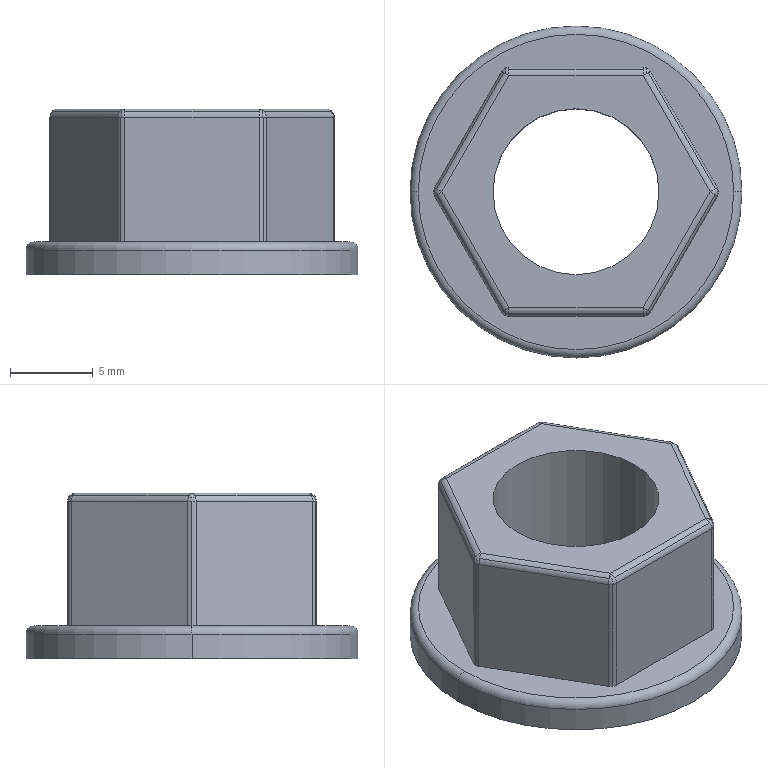Part | SolidWorks | features BaseBody 1 | 1 solid | 51 faces | box 20 x 20 x 10 mm | volume 1395 mm3 | cylinder 28 | sphere 12 | plane 9 | torus 2 | commonest cylinder face diameters 1 x24 10 x2 20 x2
STEP:
#1=CARTESIAN_POINT('',(-5.,0.,10.));
#2=VERTEX_POINT('',#1);
#3=CARTESIAN_POINT('',(5.,0.,10.));
#4=VERTEX_POINT('',#3);
#5=CARTESIAN_POINT('',(0.,0.,10.));
#6=DIRECTION('',(0.,0.,-1.));
#7=DIRECTION('',(1.,0.,0.));
#8=AXIS2_PLACEMENT_3D('',#5,#6,#7);
#9=CIRCLE('',#8,5.);
#10=EDGE_CURVE('',#2,#4,#9,.T.);
#11=ORIENTED_EDGE('',*,*,#10,.F.);
#12=CARTESIAN_POINT('',(-5.,0.,0.));
#13=VERTEX_POINT('',#12);
#14=CARTESIAN_POINT('',(-5.,0.,0.));
#15=DIRECTION('',(0.,0.,-1.));
#16=VECTOR('',#15,1000.);
#17=LINE('',#14,#16);
#18=EDGE_CURVE('',#2,#13,#17,.T.);
#19=ORIENTED_EDGE('',*,*,#18,.T.);
#20=CARTESIAN_POINT('',(5.,0.,0.));
#21=VERTEX_POINT('',#20);
#22=CARTESIAN_POINT('',(0.,0.,0.));
#23=DIRECTION('',(0.,0.,1.));
#24=DIRECTION('',(1.,0.,0.));
#25=AXIS2_PLACEMENT_3D('',#22,#23,#24);
#26=CIRCLE('',#25,5.);
#27=EDGE_CURVE('',#21,#13,#26,.T.);
#28=ORIENTED_EDGE('',*,*,#27,.F.);
#29=CARTESIAN_POINT('',(5.,0.,0.));
#30=DIRECTION('',(0.,0.,-1.));
#31=VECTOR('',#30,1000.);
#32=LINE('',#29,#31);
#33=EDGE_CURVE('',#4,#21,#32,.T.);
#34=ORIENTED_EDGE('',*,*,#33,.F.);
#35=EDGE_LOOP('',(#11,#19,#28,#34));
#36=FACE_OUTER_BOUND('',#35,.T.);
#37=CARTESIAN_POINT('',(0.,0.,0.));
#38=DIRECTION('',(0.,0.,-1.));
#39=DIRECTION('',(1.,0.,0.));
#40=AXIS2_PLACEMENT_3D('',#37,#38,#39);
#41=CYLINDRICAL_SURFACE('',#40,5.);
#42=ADVANCED_FACE('',(#36),#41,.F.);
#43=CARTESIAN_POINT('',(-4.227,-7.464,9.5));
#44=VERTEX_POINT('',#43);
#45=CARTESIAN_POINT('',(-4.291,-7.433,9.5));
#46=VERTEX_POINT('',#45);
#47=CARTESIAN_POINT('',(-4.041,-7.,9.5));
#48=DIRECTION('',(0.,0.,-1.));
#49=DIRECTION('',(0.,-1.,0.));
#50=AXIS2_PLACEMENT_3D('',#47,#48,#49);
#51=CIRCLE('',#50,0.5);
#52=EDGE_CURVE('',#44,#46,#51,.T.);
#53=ORIENTED_EDGE('',*,*,#52,.F.);
#54=CARTESIAN_POINT('',(-4.202,-7.093,9.964));
#55=VERTEX_POINT('',#54);
#56=CARTESIAN_POINT('',(-4.041,-7.,9.5));
#57=DIRECTION('',(-0.9014,0.3603,-0.2402));
#58=DIRECTION('',(-0.3712,-0.9286,0.));
#59=AXIS2_PLACEMENT_3D('',#56,#57,#58);
#60=CIRCLE('',#59,0.5);
#61=EDGE_CURVE('',#44,#55,#60,.T.);
#62=ORIENTED_EDGE('',*,*,#61,.T.);
#63=CARTESIAN_POINT('',(-4.348,-7.177,9.854));
#64=VERTEX_POINT('',#63);
#65=CARTESIAN_POINT('',(-4.041,-7.,9.5));
#66=DIRECTION('',(-0.5,0.866,0.));
#67=DIRECTION('',(-0.866,-0.5,0.));
#68=AXIS2_PLACEMENT_3D('',#65,#66,#67);
#69=CIRCLE('',#68,0.5);
#70=EDGE_CURVE('',#64,#55,#69,.T.);
#71=ORIENTED_EDGE('',*,*,#70,.F.);
#72=CARTESIAN_POINT('',(-4.474,-7.25,9.5));
#73=VERTEX_POINT('',#72);
#74=CARTESIAN_POINT('',(-4.041,-7.,9.5));
#75=DIRECTION('',(-0.5,0.866,0.));
#76=DIRECTION('',(-0.866,-0.5,0.));
#77=AXIS2_PLACEMENT_3D('',#74,#75,#76);
#78=CIRCLE('',#77,0.5);
#79=EDGE_CURVE('',#73,#64,#78,.T.);
#80=ORIENTED_EDGE('',*,*,#79,.F.);
#81=CARTESIAN_POINT('',(-4.041,-7.,9.5));
#82=DIRECTION('',(0.,0.,-1.));
#83=DIRECTION('',(0.,-1.,0.));
#84=AXIS2_PLACEMENT_3D('',#81,#82,#83);
#85=CIRCLE('',#84,0.5);
#86=EDGE_CURVE('',#46,#73,#85,.T.);
#87=ORIENTED_EDGE('',*,*,#86,.F.);
#88=EDGE_LOOP('',(#53,#62,#71,#80,#87));
#89=FACE_OUTER_BOUND('',#88,.T.);
#90=CARTESIAN_POINT('',(-4.041,-7.,9.5));
#91=DIRECTION('',(0.9014,-0.3603,0.2402));
#92=DIRECTION('',(-0.433,-0.75,0.5));
#93=AXIS2_PLACEMENT_3D('',#90,#91,#92);
#94=SPHERICAL_SURFACE('',#93,0.5);
#95=ADVANCED_FACE('',(#89),#94,.T.);
#96=CARTESIAN_POINT('',(-4.041,-7.5,9.5));
#97=VERTEX_POINT('',#96);
#98=CARTESIAN_POINT('',(-4.041,-7.,9.5));
#99=DIRECTION('',(0.,0.,-1.));
#100=DIRECTION('',(0.,-1.,0.));
#101=AXIS2_PLACEMENT_3D('',#98,#99,#100);
#102=CIRCLE('',#101,0.5);
#103=EDGE_CURVE('',#97,#44,#102,.T.);
#104=ORIENTED_EDGE('',*,*,#103,.T.);
#105=ORIENTED_EDGE('',*,*,#52,.T.);
#106=CARTESIAN_POINT('',(-4.291,-7.433,2.));
#107=VERTEX_POINT('',#106);
#108=CARTESIAN_POINT('',(-4.291,-7.433,2.));
#109=DIRECTION('',(0.,0.,-1.));
#110=VECTOR('',#109,1000.);
#111=LINE('',#108,#110);
#112=EDGE_CURVE('',#46,#107,#111,.T.);
#113=ORIENTED_EDGE('',*,*,#112,.T.);
#114=CARTESIAN_POINT('',(-4.041,-7.5,2.));
#115=VERTEX_POINT('',#114);
#116=CARTESIAN_POINT('',(-4.041,-7.,2.));
#117=DIRECTION('',(0.,0.,1.));
#118=DIRECTION('',(-0.5,-0.866,0.));
#119=AXIS2_PLACEMENT_3D('',#116,#117,#118);
#120=CIRCLE('',#119,0.5);
#121=EDGE_CURVE('',#107,#115,#120,.T.);
#122=ORIENTED_EDGE('',*,*,#121,.T.);
#123=CARTESIAN_POINT('',(-4.041,-7.5,2.));
#124=DIRECTION('',(0.,0.,1.));
#125=VECTOR('',#124,1000.);
#126=LINE('',#123,#125);
#127=EDGE_CURVE('',#115,#97,#126,.T.);
#128=ORIENTED_EDGE('',*,*,#127,.T.);
#129=EDGE_LOOP('',(#104,#105,#113,#122,#128));
#130=FACE_OUTER_BOUND('',#129,.T.);
#131=CARTESIAN_POINT('',(-4.041,-7.,2.));
#132=DIRECTION('',(0.,0.,-1.));
#133=DIRECTION('',(-0.5,-0.866,0.));
#134=AXIS2_PLACEMENT_3D('',#131,#132,#133);
#135=CYLINDRICAL_SURFACE('',#134,0.5);
#136=ADVANCED_FACE('',(#130),#135,.T.);
#137=CARTESIAN_POINT('',(4.227,-7.464,9.5));
#138=VERTEX_POINT('',#137);
#139=CARTESIAN_POINT('',(4.041,-7.5,9.5));
#140=VERTEX_POINT('',#139);
#141=CARTESIAN_POINT('',(4.041,-7.,9.5));
#142=DIRECTION('',(0.,0.,-1.));
#143=DIRECTION('',(0.866,-0.5,0.));
#144=AXIS2_PLACEMENT_3D('',#141,#142,#143);
#145=CIRCLE('',#144,0.5);
#146=EDGE_CURVE('',#138,#140,#145,.T.);
#147=ORIENTED_EDGE('',*,*,#146,.F.);
#148=CARTESIAN_POINT('',(4.202,-7.093,9.964));
#149=VERTEX_POINT('',#148);
#150=CARTESIAN_POINT('',(4.041,-7.,9.5));
#151=DIRECTION('',(-0.9014,-0.3603,0.2402));
#152=DIRECTION('',(0.3712,-0.9286,0.));
#153=AXIS2_PLACEMENT_3D('',#150,#151,#152);
#154=CIRCLE('',#153,0.5);
#155=EDGE_CURVE('',#138,#149,#154,.T.);
#156=ORIENTED_EDGE('',*,*,#155,.T.);
#157=CARTESIAN_POINT('',(4.041,-7.,10.));
#158=VERTEX_POINT('',#157);
#159=CARTESIAN_POINT('',(4.041,-7.,9.5));
#160=DIRECTION('',(0.5,0.866,0.));
#161=DIRECTION('',(0.,0.,1.));
#162=AXIS2_PLACEMENT_3D('',#159,#160,#161);
#163=CIRCLE('',#162,0.5);
#164=EDGE_CURVE('',#158,#149,#163,.T.);
#165=ORIENTED_EDGE('',*,*,#164,.F.);
#166=CARTESIAN_POINT('',(4.041,-7.354,9.854));
#167=VERTEX_POINT('',#166);
#168=CARTESIAN_POINT('',(4.041,-7.,9.5));
#169=DIRECTION('',(-1.,0.,0.));
#170=DIRECTION('',(0.,-1.,0.));
#171=AXIS2_PLACEMENT_3D('',#168,#169,#170);
#172=CIRCLE('',#171,0.5);
#173=EDGE_CURVE('',#167,#158,#172,.T.);
#174=ORIENTED_EDGE('',*,*,#173,.F.);
#175=CARTESIAN_POINT('',(4.041,-7.,9.5));
#176=DIRECTION('',(-1.,0.,0.));
#177=DIRECTION('',(0.,-1.,0.));
#178=AXIS2_PLACEMENT_3D('',#175,#176,#177);
#179=CIRCLE('',#178,0.5);
#180=EDGE_CURVE('',#140,#167,#179,.T.);
#181=ORIENTED_EDGE('',*,*,#180,.F.);
#182=EDGE_LOOP('',(#147,#156,#165,#174,#181));
#183=FACE_OUTER_BOUND('',#182,.T.);
#184=CARTESIAN_POINT('',(4.041,-7.,9.5));
#185=DIRECTION('',(0.9014,0.3603,-0.2402));
#186=DIRECTION('',(0.433,-0.75,0.5));
#187=AXIS2_PLACEMENT_3D('',#184,#185,#186);
#188=SPHERICAL_SURFACE('',#187,0.5);
#189=ADVANCED_FACE('',(#183),#188,.T.);
#190=CARTESIAN_POINT('',(4.474,-7.25,9.5));
#191=VERTEX_POINT('',#190);
#192=CARTESIAN_POINT('',(4.291,-7.433,9.5));
#193=VERTEX_POINT('',#192);
#194=CARTESIAN_POINT('',(4.041,-7.,9.5));
#195=DIRECTION('',(0.,0.,-1.));
#196=DIRECTION('',(0.866,-0.5,0.));
#197=AXIS2_PLACEMENT_3D('',#194,#195,#196);
#198=CIRCLE('',#197,0.5);
#199=EDGE_CURVE('',#191,#193,#198,.T.);
#200=ORIENTED_EDGE('',*,*,#199,.T.);
#201=CARTESIAN_POINT('',(4.291,-7.433,2.));
#202=VERTEX_POINT('',#201);
#203=CARTESIAN_POINT('',(4.291,-7.433,2.));
#204=DIRECTION('',(0.,0.,-1.));
#205=VECTOR('',#204,1000.);
#206=LINE('',#203,#205);
#207=EDGE_CURVE('',#193,#202,#206,.T.);
#208=ORIENTED_EDGE('',*,*,#207,.T.);
#209=CARTESIAN_POINT('',(4.474,-7.25,2.));
#210=VERTEX_POINT('',#209);
#211=CARTESIAN_POINT('',(4.041,-7.,2.));
#212=DIRECTION('',(0.,0.,1.));
#213=DIRECTION('',(0.5,-0.866,0.));
#214=AXIS2_PLACEMENT_3D('',#211,#212,#213);
#215=CIRCLE('',#214,0.5);
#216=EDGE_CURVE('',#202,#210,#215,.T.);
#217=ORIENTED_EDGE('',*,*,#216,.T.);
#218=CARTESIAN_POINT('',(4.474,-7.25,2.));
#219=DIRECTION('',(0.,0.,1.));
#220=VECTOR('',#219,1000.);
#221=LINE('',#218,#220);
#222=EDGE_CURVE('',#210,#191,#221,.T.);
#223=ORIENTED_EDGE('',*,*,#222,.T.);
#224=EDGE_LOOP('',(#200,#208,#217,#223));
#225=FACE_OUTER_BOUND('',#224,.T.);
#226=CARTESIAN_POINT('',(4.041,-7.,2.));
#227=DIRECTION('',(0.,0.,-1.));
#228=DIRECTION('',(0.5,-0.866,0.));
#229=AXIS2_PLACEMENT_3D('',#226,#227,#228);
#230=CYLINDRICAL_SURFACE('',#229,0.5);
#231=ADVANCED_FACE('',(#225),#230,.T.);
#232=CARTESIAN_POINT('',(-8.47,-0.2236,9.724));
#233=VERTEX_POINT('',#232);
#234=CARTESIAN_POINT('',(-8.516,-0.25,9.5));
#235=VERTEX_POINT('',#234);
#236=CARTESIAN_POINT('',(-8.083,0.,9.5));
#237=DIRECTION('',(0.5,-0.866,0.));
#238=DIRECTION('',(0.,0.,1.));
#239=AXIS2_PLACEMENT_3D('',#236,#237,#238);
#240=CIRCLE('',#239,0.5);
#241=EDGE_CURVE('',#233,#235,#240,.T.);
#242=ORIENTED_EDGE('',*,*,#241,.F.);
#243=CARTESIAN_POINT('',(-8.47,0.2236,9.724));
#244=VERTEX_POINT('',#243);
#245=CARTESIAN_POINT('',(-8.083,0.,9.5));
#246=DIRECTION('',(-0.5,0.,-0.866));
#247=DIRECTION('',(-0.866,0.,0.5));
#248=AXIS2_PLACEMENT_3D('',#245,#246,#247);
#249=CIRCLE('',#248,0.5);
#250=EDGE_CURVE('',#233,#244,#249,.T.);
#251=ORIENTED_EDGE('',*,*,#250,.T.);
#252=CARTESIAN_POINT('',(-8.516,0.25,9.5));
#253=VERTEX_POINT('',#252);
#254=CARTESIAN_POINT('',(-8.083,0.,9.5));
#255=DIRECTION('',(0.5,0.866,0.));
#256=DIRECTION('',(-0.866,0.5,0.));
#257=AXIS2_PLACEMENT_3D('',#254,#255,#256);
#258=CIRCLE('',#257,0.5);
#259=EDGE_CURVE('',#253,#244,#258,.T.);
#260=ORIENTED_EDGE('',*,*,#259,.F.);
#261=CARTESIAN_POINT('',(-8.583,0.,9.5));
#262=VERTEX_POINT('',#261);
#263=CARTESIAN_POINT('',(-8.083,0.,9.5));
#264=DIRECTION('',(0.,0.,-1.));
#265=DIRECTION('',(-0.866,-0.5,0.));
#266=AXIS2_PLACEMENT_3D('',#263,#264,#265);
#267=CIRCLE('',#266,0.5);
#268=EDGE_CURVE('',#262,#253,#267,.T.);
#269=ORIENTED_EDGE('',*,*,#268,.F.);
#270=CARTESIAN_POINT('',(-8.083,0.,9.5));
#271=DIRECTION('',(0.,0.,-1.));
#272=DIRECTION('',(-0.866,-0.5,0.));
#273=AXIS2_PLACEMENT_3D('',#270,#271,#272);
#274=CIRCLE('',#273,0.5);
#275=EDGE_CURVE('',#235,#262,#274,.T.);
#276=ORIENTED_EDGE('',*,*,#275,.F.);
#277=EDGE_LOOP('',(#242,#251,#260,#269,#276));
#278=FACE_OUTER_BOUND('',#277,.T.);
#279=CARTESIAN_POINT('',(-8.083,0.,9.5));
#280=DIRECTION('',(0.5,0.,0.866));
#281=DIRECTION('',(-0.866,0.,0.5));
#282=AXIS2_PLACEMENT_3D('',#279,#280,#281);
#283=SPHERICAL_SURFACE('',#282,0.5);
#284=ADVANCED_FACE('',(#278),#283,.T.);
#285=ORIENTED_EDGE('',*,*,#275,.T.);
#286=CARTESIAN_POINT('',(-8.583,0.,2.));
#287=VERTEX_POINT('',#286);
#288=CARTESIAN_POINT('',(-8.583,0.,2.));
#289=DIRECTION('',(0.,0.,-1.));
#290=VECTOR('',#289,1000.);
#291=LINE('',#288,#290);
#292=EDGE_CURVE('',#262,#287,#291,.T.);
#293=ORIENTED_EDGE('',*,*,#292,.T.);
#294=CARTESIAN_POINT('',(-8.516,-0.25,2.));
#295=VERTEX_POINT('',#294);
#296=CARTESIAN_POINT('',(-8.083,0.,2.));
#297=DIRECTION('',(0.,0.,1.));
#298=DIRECTION('',(-1.,0.,0.));
#299=AXIS2_PLACEMENT_3D('',#296,#297,#298);
#300=CIRCLE('',#299,0.5);
#301=EDGE_CURVE('',#287,#295,#300,.T.);
#302=ORIENTED_EDGE('',*,*,#301,.T.);
#303=CARTESIAN_POINT('',(-8.516,-0.25,2.));
#304=DIRECTION('',(0.,0.,1.));
#305=VECTOR('',#304,1000.);
#306=LINE('',#303,#305);
#307=EDGE_CURVE('',#295,#235,#306,.T.);
#308=ORIENTED_EDGE('',*,*,#307,.T.);
#309=EDGE_LOOP('',(#285,#293,#302,#308));
#310=FACE_OUTER_BOUND('',#309,.T.);
#311=CARTESIAN_POINT('',(-8.083,0.,2.));
#312=DIRECTION('',(0.,0.,-1.));
#313=DIRECTION('',(-1.,0.,0.));
#314=AXIS2_PLACEMENT_3D('',#311,#312,#313);
#315=CYLINDRICAL_SURFACE('',#314,0.5);
#316=ADVANCED_FACE('',(#310),#315,.T.);
#317=ORIENTED_EDGE('',*,*,#79,.T.);
#318=CARTESIAN_POINT('',(-8.389,-0.1768,9.854));
#319=VERTEX_POINT('',#318);
#320=CARTESIAN_POINT('',(-7.451,-1.802,9.854));
#321=DIRECTION('',(-0.5,0.866,0.));
#322=VECTOR('',#321,1000.);
#323=LINE('',#320,#322);
#324=EDGE_CURVE('',#64,#319,#323,.T.);
#325=ORIENTED_EDGE('',*,*,#324,.T.);
#326=CARTESIAN_POINT('',(-8.083,0.,9.5));
#327=DIRECTION('',(0.5,-0.866,0.));
#328=DIRECTION('',(0.,0.,1.));
#329=AXIS2_PLACEMENT_3D('',#326,#327,#328);
#330=CIRCLE('',#329,0.5);
#331=EDGE_CURVE('',#319,#233,#330,.T.);
#332=ORIENTED_EDGE('',*,*,#331,.T.);
#333=ORIENTED_EDGE('',*,*,#241,.T.);
#334=CARTESIAN_POINT('',(-7.578,-1.875,9.5));
#335=DIRECTION('',(0.5,-0.866,0.));
#336=VECTOR('',#335,1000.);
#337=LINE('',#334,#336);
#338=EDGE_CURVE('',#235,#73,#337,.T.);
#339=ORIENTED_EDGE('',*,*,#338,.T.);
#340=EDGE_LOOP('',(#317,#325,#332,#333,#339));
#341=FACE_OUTER_BOUND('',#340,.T.);
#342=CARTESIAN_POINT('',(-7.145,-1.625,9.5));
#343=DIRECTION('',(-0.5,0.866,0.));
#344=DIRECTION('',(-0.6124,-0.3536,0.7071));
#345=AXIS2_PLACEMENT_3D('',#342,#343,#344);
#346=CYLINDRICAL_SURFACE('',#345,0.5);
#347=ADVANCED_FACE('',(#341),#346,.T.);
#348=CARTESIAN_POINT('',(8.47,0.2236,9.724));
#349=VERTEX_POINT('',#348);
#350=CARTESIAN_POINT('',(8.516,0.25,9.5));
#351=VERTEX_POINT('',#350);
#352=CARTESIAN_POINT('',(8.083,0.,9.5));
#353=DIRECTION('',(-0.5,0.866,0.));
#354=DIRECTION('',(0.,0.,1.));
#355=AXIS2_PLACEMENT_3D('',#352,#353,#354);
#356=CIRCLE('',#355,0.5);
#357=EDGE_CURVE('',#349,#351,#356,.T.);
#358=ORIENTED_EDGE('',*,*,#357,.F.);
#359=CARTESIAN_POINT('',(8.47,-0.2236,9.724));
#360=VERTEX_POINT('',#359);
#361=CARTESIAN_POINT('',(8.083,0.,9.5));
#362=DIRECTION('',(0.5,0.,-0.866));
#363=DIRECTION('',(-0.866,0.,-0.5));
#364=AXIS2_PLACEMENT_3D('',#361,#362,#363);
#365=CIRCLE('',#364,0.5);
#366=EDGE_CURVE('',#349,#360,#365,.T.);
#367=ORIENTED_EDGE('',*,*,#366,.T.);
#368=CARTESIAN_POINT('',(8.516,-0.25,9.5));
#369=VERTEX_POINT('',#368);
#370=CARTESIAN_POINT('',(8.083,0.,9.5));
#371=DIRECTION('',(-0.5,-0.866,0.));
#372=DIRECTION('',(0.866,-0.5,0.));
#373=AXIS2_PLACEMENT_3D('',#370,#371,#372);
#374=CIRCLE('',#373,0.5);
#375=EDGE_CURVE('',#369,#360,#374,.T.);
#376=ORIENTED_EDGE('',*,*,#375,.F.);
#377=CARTESIAN_POINT('',(8.583,0.,9.5));
#378=VERTEX_POINT('',#377);
#379=CARTESIAN_POINT('',(8.083,0.,9.5));
#380=DIRECTION('',(0.,0.,-1.));
#381=DIRECTION('',(0.866,0.5,0.));
#382=AXIS2_PLACEMENT_3D('',#379,#380,#381);
#383=CIRCLE('',#382,0.5);
#384=EDGE_CURVE('',#378,#369,#383,.T.);
#385=ORIENTED_EDGE('',*,*,#384,.F.);
#386=CARTESIAN_POINT('',(8.083,0.,9.5));
#387=DIRECTION('',(0.,0.,-1.));
#388=DIRECTION('',(0.866,0.5,0.));
#389=AXIS2_PLACEMENT_3D('',#386,#387,#388);
#390=CIRCLE('',#389,0.5);
#391=EDGE_CURVE('',#351,#378,#390,.T.);
#392=ORIENTED_EDGE('',*,*,#391,.F.);
#393=EDGE_LOOP('',(#358,#367,#376,#385,#392));
#394=FACE_OUTER_BOUND('',#393,.T.);
#395=CARTESIAN_POINT('',(8.083,0.,9.5));
#396=DIRECTION('',(-0.5,0.,0.866));
#397=DIRECTION('',(0.866,0.,0.5));
#398=AXIS2_PLACEMENT_3D('',#395,#396,#397);
#399=SPHERICAL_SURFACE('',#398,0.5);
#400=ADVANCED_FACE('',(#394),#399,.T.);
#401=ORIENTED_EDGE('',*,*,#391,.T.);
#402=CARTESIAN_POINT('',(8.583,0.,2.));
#403=VERTEX_POINT('',#402);
#404=CARTESIAN_POINT('',(8.583,0.,2.));
#405=DIRECTION('',(0.,0.,-1.));
#406=VECTOR('',#405,1000.);
#407=LINE('',#404,#406);
#408=EDGE_CURVE('',#378,#403,#407,.T.);
#409=ORIENTED_EDGE('',*,*,#408,.T.);
#410=CARTESIAN_POINT('',(8.516,0.25,2.));
#411=VERTEX_POINT('',#410);
#412=CARTESIAN_POINT('',(8.083,0.,2.));
#413=DIRECTION('',(0.,0.,1.));
#414=DIRECTION('',(1.,0.,0.));
#415=AXIS2_PLACEMENT_3D('',#412,#413,#414);
#416=CIRCLE('',#415,0.5);
#417=EDGE_CURVE('',#403,#411,#416,.T.);
#418=ORIENTED_EDGE('',*,*,#417,.T.);
#419=CARTESIAN_POINT('',(8.516,0.25,2.));
#420=DIRECTION('',(0.,0.,1.));
#421=VECTOR('',#420,1000.);
#422=LINE('',#419,#421);
#423=EDGE_CURVE('',#411,#351,#422,.T.);
#424=ORIENTED_EDGE('',*,*,#423,.T.);
#425=EDGE_LOOP('',(#401,#409,#418,#424));
#426=FACE_OUTER_BOUND('',#425,.T.);
#427=CARTESIAN_POINT('',(8.083,0.,2.));
#428=DIRECTION('',(0.,0.,-1.));
#429=DIRECTION('',(1.,0.,0.));
#430=AXIS2_PLACEMENT_3D('',#427,#428,#429);
#431=CYLINDRICAL_SURFACE('',#430,0.5);
#432=ADVANCED_FACE('',(#426),#431,.T.);
#433=CARTESIAN_POINT('',(-4.202,7.093,9.964));
#434=VERTEX_POINT('',#433);
#435=CARTESIAN_POINT('',(-4.348,7.177,9.854));
#436=VERTEX_POINT('',#435);
#437=CARTESIAN_POINT('',(-4.041,7.,9.5));
#438=DIRECTION('',(-0.5,-0.866,0.));
#439=DIRECTION('',(0.,0.,1.));
#440=AXIS2_PLACEMENT_3D('',#437,#438,#439);
#441=CIRCLE('',#440,0.5);
#442=EDGE_CURVE('',#434,#436,#441,.T.);
#443=ORIENTED_EDGE('',*,*,#442,.F.);
#444=CARTESIAN_POINT('',(-4.227,7.464,9.5));
#445=VERTEX_POINT('',#444);
#446=CARTESIAN_POINT('',(-4.041,7.,9.5));
#447=DIRECTION('',(-0.9014,-0.3603,-0.2402));
#448=DIRECTION('',(0.3712,-0.9286,0.));
#449=AXIS2_PLACEMENT_3D('',#446,#447,#448);
#450=CIRCLE('',#449,0.5);
#451=EDGE_CURVE('',#434,#445,#450,.T.);
#452=ORIENTED_EDGE('',*,*,#451,.T.);
#453=CARTESIAN_POINT('',(-4.291,7.433,9.5));
#454=VERTEX_POINT('',#453);
#455=CARTESIAN_POINT('',(-4.041,7.,9.5));
#456=DIRECTION('',(0.,0.,-1.));
#457=DIRECTION('',(-0.866,0.5,0.));
#458=AXIS2_PLACEMENT_3D('',#455,#456,#457);
#459=CIRCLE('',#458,0.5);
#460=EDGE_CURVE('',#454,#445,#459,.T.);
#461=ORIENTED_EDGE('',*,*,#460,.F.);
#462=CARTESIAN_POINT('',(-4.474,7.25,9.5));
#463=VERTEX_POINT('',#462);
#464=CARTESIAN_POINT('',(-4.041,7.,9.5));
#465=DIRECTION('',(0.,0.,-1.));
#466=DIRECTION('',(-0.866,0.5,0.));
#467=AXIS2_PLACEMENT_3D('',#464,#465,#466);
#468=CIRCLE('',#467,0.5);
#469=EDGE_CURVE('',#463,#454,#468,.T.);
#470=ORIENTED_EDGE('',*,*,#469,.F.);
#471=CARTESIAN_POINT('',(-4.041,7.,9.5));
#472=DIRECTION('',(-0.5,-0.866,0.));
#473=DIRECTION('',(0.,0.,1.));
#474=AXIS2_PLACEMENT_3D('',#471,#472,#473);
#475=CIRCLE('',#474,0.5);
#476=EDGE_CURVE('',#436,#463,#475,.T.);
#477=ORIENTED_EDGE('',*,*,#476,.F.);
#478=EDGE_LOOP('',(#443,#452,#461,#470,#477));
#479=FACE_OUTER_BOUND('',#478,.T.);
#480=CARTESIAN_POINT('',(-4.041,7.,9.5));
#481=DIRECTION('',(0.9014,0.3603,0.2402));
#482=DIRECTION('',(-0.433,0.75,0.5));
#483=AXIS2_PLACEMENT_3D('',#480,#481,#482);
#484=SPHERICAL_SURFACE('',#483,0.5);
#485=ADVANCED_FACE('',(#479),#484,.T.);
#486=ORIENTED_EDGE('',*,*,#469,.T.);
#487=CARTESIAN_POINT('',(-4.291,7.433,2.));
#488=VERTEX_POINT('',#487);
#489=CARTESIAN_POINT('',(-4.291,7.433,2.));
#490=DIRECTION('',(0.,0.,-1.));
#491=VECTOR('',#490,1000.);
#492=LINE('',#489,#491);
#493=EDGE_CURVE('',#454,#488,#492,.T.);
#494=ORIENTED_EDGE('',*,*,#493,.T.);
#495=CARTESIAN_POINT('',(-4.474,7.25,2.));
#496=VERTEX_POINT('',#495);
#497=CARTESIAN_POINT('',(-4.041,7.,2.));
#498=DIRECTION('',(0.,0.,1.));
#499=DIRECTION('',(-0.5,0.866,0.));
#500=AXIS2_PLACEMENT_3D('',#497,#498,#499);
#501=CIRCLE('',#500,0.5);
#502=EDGE_CURVE('',#488,#496,#501,.T.);
#503=ORIENTED_EDGE('',*,*,#502,.T.);
#504=CARTESIAN_POINT('',(-4.474,7.25,2.));
#505=DIRECTION('',(0.,0.,1.));
#506=VECTOR('',#505,1000.);
#507=LINE('',#504,#506);
#508=EDGE_CURVE('',#496,#463,#507,.T.);
#509=ORIENTED_EDGE('',*,*,#508,.T.);
#510=EDGE_LOOP('',(#486,#494,#503,#509));
#511=FACE_OUTER_BOUND('',#510,.T.);
#512=CARTESIAN_POINT('',(-4.041,7.,2.));
#513=DIRECTION('',(0.,0.,-1.));
#514=DIRECTION('',(-0.5,0.866,0.));
#515=AXIS2_PLACEMENT_3D('',#512,#513,#514);
#516=CYLINDRICAL_SURFACE('',#515,0.5);
#517=ADVANCED_FACE('',(#511),#516,.T.);
#518=ORIENTED_EDGE('',*,*,#259,.T.);
#519=CARTESIAN_POINT('',(-8.389,0.1768,9.854));
#520=VERTEX_POINT('',#519);
#521=CARTESIAN_POINT('',(-8.083,0.,9.5));
#522=DIRECTION('',(0.5,0.866,0.));
#523=DIRECTION('',(-0.866,0.5,0.));
#524=AXIS2_PLACEMENT_3D('',#521,#522,#523);
#525=CIRCLE('',#524,0.5);
#526=EDGE_CURVE('',#244,#520,#525,.T.);
#527=ORIENTED_EDGE('',*,*,#526,.T.);
#528=CARTESIAN_POINT('',(-5.286,5.552,9.854));
#529=DIRECTION('',(0.5,0.866,0.));
#530=VECTOR('',#529,1000.);
#531=LINE('',#528,#530);
#532=EDGE_CURVE('',#520,#436,#531,.T.);
#533=ORIENTED_EDGE('',*,*,#532,.T.);
#534=ORIENTED_EDGE('',*,*,#476,.T.);
#535=CARTESIAN_POINT('',(-5.413,5.625,9.5));
#536=DIRECTION('',(-0.5,-0.866,0.));
#537=VECTOR('',#536,1000.);
#538=LINE('',#535,#537);
#539=EDGE_CURVE('',#463,#253,#538,.T.);
#540=ORIENTED_EDGE('',*,*,#539,.T.);
#541=EDGE_LOOP('',(#518,#527,#533,#534,#540));
#542=FACE_OUTER_BOUND('',#541,.T.);
#543=CARTESIAN_POINT('',(-4.98,5.375,9.5));
#544=DIRECTION('',(0.5,0.866,0.));
#545=DIRECTION('',(-0.6124,0.3536,0.7071));
#546=AXIS2_PLACEMENT_3D('',#543,#544,#545);
#547=CYLINDRICAL_SURFACE('',#546,0.5);
#548=ADVANCED_FACE('',(#542),#547,.T.);
#549=CARTESIAN_POINT('',(4.202,7.093,9.964));
#550=VERTEX_POINT('',#549);
#551=CARTESIAN_POINT('',(4.041,7.,10.));
#552=VERTEX_POINT('',#551);
#553=CARTESIAN_POINT('',(4.041,7.,9.5));
#554=DIRECTION('',(0.5,-0.866,0.));
#555=DIRECTION('',(0.866,0.5,0.));
#556=AXIS2_PLACEMENT_3D('',#553,#554,#555);
#557=CIRCLE('',#556,0.5);
#558=EDGE_CURVE('',#550,#552,#557,.T.);
#559=ORIENTED_EDGE('',*,*,#558,.F.);
#560=CARTESIAN_POINT('',(4.227,7.464,9.5));
#561=VERTEX_POINT('',#560);
#562=CARTESIAN_POINT('',(4.041,7.,9.5));
#563=DIRECTION('',(-0.9014,0.3603,0.2402));
#564=DIRECTION('',(-0.3712,-0.9286,0.));
#565=AXIS2_PLACEMENT_3D('',#562,#563,#564);
#566=CIRCLE('',#565,0.5);
#567=EDGE_CURVE('',#550,#561,#566,.T.);
#568=ORIENTED_EDGE('',*,*,#567,.T.);
#569=CARTESIAN_POINT('',(4.041,7.5,9.5));
#570=VERTEX_POINT('',#569);
#571=CARTESIAN_POINT('',(4.041,7.,9.5));
#572=DIRECTION('',(0.,0.,-1.));
#573=DIRECTION('',(0.,1.,0.));
#574=AXIS2_PLACEMENT_3D('',#571,#572,#573);
#575=CIRCLE('',#574,0.5);
#576=EDGE_CURVE('',#570,#561,#575,.T.);
#577=ORIENTED_EDGE('',*,*,#576,.F.);
#578=CARTESIAN_POINT('',(4.041,7.354,9.854));
#579=VERTEX_POINT('',#578);
#580=CARTESIAN_POINT('',(4.041,7.,9.5));
#581=DIRECTION('',(-1.,0.,0.));
#582=DIRECTION('',(0.,0.,1.));
#583=AXIS2_PLACEMENT_3D('',#580,#581,#582);
#584=CIRCLE('',#583,0.5);
#585=EDGE_CURVE('',#579,#570,#584,.T.);
#586=ORIENTED_EDGE('',*,*,#585,.F.);
#587=CARTESIAN_POINT('',(4.041,7.,9.5));
#588=DIRECTION('',(-1.,0.,0.));
#589=DIRECTION('',(0.,0.,1.));
#590=AXIS2_PLACEMENT_3D('',#587,#588,#589);
#591=CIRCLE('',#590,0.5);
#592=EDGE_CURVE('',#552,#579,#591,.T.);
#593=ORIENTED_EDGE('',*,*,#592,.F.);
#594=EDGE_LOOP('',(#559,#568,#577,#586,#593));
#595=FACE_OUTER_BOUND('',#594,.T.);
#596=CARTESIAN_POINT('',(4.041,7.,9.5));
#597=DIRECTION('',(0.9014,-0.3603,-0.2402));
#598=DIRECTION('',(0.433,0.75,0.5));
#599=AXIS2_PLACEMENT_3D('',#596,#597,#598);
#600=SPHERICAL_SURFACE('',#599,0.5);
#601=ADVANCED_FACE('',(#595),#600,.T.);
#602=ORIENTED_EDGE('',*,*,#576,.T.);
#603=CARTESIAN_POINT('',(4.291,7.433,9.5));
#604=VERTEX_POINT('',#603);
#605=CARTESIAN_POINT('',(4.041,7.,9.5));
#606=DIRECTION('',(0.,0.,-1.));
#607=DIRECTION('',(0.,1.,0.));
#608=AXIS2_PLACEMENT_3D('',#605,#606,#607);
#609=CIRCLE('',#608,0.5);
#610=EDGE_CURVE('',#561,#604,#609,.T.);
#611=ORIENTED_EDGE('',*,*,#610,.T.);
#612=CARTESIAN_POINT('',(4.291,7.433,2.));
#613=VERTEX_POINT('',#612);
#614=CARTESIAN_POINT('',(4.291,7.433,2.));
#615=DIRECTION('',(0.,0.,-1.));
#616=VECTOR('',#615,1000.);
#617=LINE('',#614,#616);
#618=EDGE_CURVE('',#604,#613,#617,.T.);
#619=ORIENTED_EDGE('',*,*,#618,.T.);
#620=CARTESIAN_POINT('',(4.041,7.5,2.));
#621=VERTEX_POINT('',#620);
#622=CARTESIAN_POINT('',(4.041,7.,2.));
#623=DIRECTION('',(0.,0.,1.));
#624=DIRECTION('',(0.5,0.866,0.));
#625=AXIS2_PLACEMENT_3D('',#622,#623,#624);
#626=CIRCLE('',#625,0.5);
#627=EDGE_CURVE('',#613,#621,#626,.T.);
#628=ORIENTED_EDGE('',*,*,#627,.T.);
#629=CARTESIAN_POINT('',(4.041,7.5,2.));
#630=DIRECTION('',(0.,0.,1.));
#631=VECTOR('',#630,1000.);
#632=LINE('',#629,#631);
#633=EDGE_CURVE('',#621,#570,#632,.T.);
#634=ORIENTED_EDGE('',*,*,#633,.T.);
#635=EDGE_LOOP('',(#602,#611,#619,#628,#634));
#636=FACE_OUTER_BOUND('',#635,.T.);
#637=CARTESIAN_POINT('',(4.041,7.,2.));
#638=DIRECTION('',(0.,0.,-1.));
#639=DIRECTION('',(0.5,0.866,0.));
#640=AXIS2_PLACEMENT_3D('',#637,#638,#639);
#641=CYLINDRICAL_SURFACE('',#640,0.5);
#642=ADVANCED_FACE('',(#636),#641,.T.);
#643=CARTESIAN_POINT('',(-4.041,7.5,9.5));
#644=VERTEX_POINT('',#643);
#645=CARTESIAN_POINT('',(-4.041,7.354,9.854));
#646=VERTEX_POINT('',#645);
#647=CARTESIAN_POINT('',(-4.041,7.,9.5));
#648=DIRECTION('',(1.,0.,0.));
#649=DIRECTION('',(0.,1.,0.));
#650=AXIS2_PLACEMENT_3D('',#647,#648,#649);
#651=CIRCLE('',#650,0.5);
#652=EDGE_CURVE('',#644,#646,#651,.T.);
#653=ORIENTED_EDGE('',*,*,#652,.T.);
#654=CARTESIAN_POINT('',(2.165,7.354,9.854));
#655=DIRECTION('',(1.,0.,0.));
#656=VECTOR('',#655,1000.);
#657=LINE('',#654,#656);
#658=EDGE_CURVE('',#646,#579,#657,.T.);
#659=ORIENTED_EDGE('',*,*,#658,.T.);
#660=ORIENTED_EDGE('',*,*,#585,.T.);
#661=CARTESIAN_POINT('',(2.165,7.5,9.5));
#662=DIRECTION('',(-1.,0.,0.));
#663=VECTOR('',#662,1000.);
#664=LINE('',#661,#663);
#665=EDGE_CURVE('',#570,#644,#664,.T.);
#666=ORIENTED_EDGE('',*,*,#665,.T.);
#667=EDGE_LOOP('',(#653,#659,#660,#666));
#668=FACE_OUTER_BOUND('',#667,.T.);
#669=CARTESIAN_POINT('',(2.165,7.,9.5));
#670=DIRECTION('',(1.,0.,0.));
#671=DIRECTION('',(0.,0.7071,0.7071));
#672=AXIS2_PLACEMENT_3D('',#669,#670,#671);
#673=CYLINDRICAL_SURFACE('',#672,0.5);
#674=ADVANCED_FACE('',(#668),#673,.T.);
#675=CARTESIAN_POINT('',(4.474,7.25,9.5));
#676=VERTEX_POINT('',#675);
#677=CARTESIAN_POINT('',(4.348,7.177,9.854));
#678=VERTEX_POINT('',#677);
#679=CARTESIAN_POINT('',(4.041,7.,9.5));
#680=DIRECTION('',(0.5,-0.866,0.));
#681=DIRECTION('',(0.866,0.5,0.));
#682=AXIS2_PLACEMENT_3D('',#679,#680,#681);
#683=CIRCLE('',#682,0.5);
#684=EDGE_CURVE('',#676,#678,#683,.T.);
#685=ORIENTED_EDGE('',*,*,#684,.T.);
#686=CARTESIAN_POINT('',(8.389,0.1768,9.854));
#687=VERTEX_POINT('',#686);
#688=CARTESIAN_POINT('',(7.451,1.802,9.854));
#689=DIRECTION('',(0.5,-0.866,0.));
#690=VECTOR('',#689,1000.);
#691=LINE('',#688,#690);
#692=EDGE_CURVE('',#678,#687,#691,.T.);
#693=ORIENTED_EDGE('',*,*,#692,.T.);
#694=CARTESIAN_POINT('',(8.083,0.,9.5));
#695=DIRECTION('',(-0.5,0.866,0.));
#696=DIRECTION('',(0.,0.,1.));
#697=AXIS2_PLACEMENT_3D('',#694,#695,#696);
#698=CIRCLE('',#697,0.5);
#699=EDGE_CURVE('',#687,#349,#698,.T.);
#700=ORIENTED_EDGE('',*,*,#699,.T.);
#701=ORIENTED_EDGE('',*,*,#357,.T.);
#702=CARTESIAN_POINT('',(7.578,1.875,9.5));
#703=DIRECTION('',(-0.5,0.866,0.));
#704=VECTOR('',#703,1000.);
#705=LINE('',#702,#704);
#706=EDGE_CURVE('',#351,#676,#705,.T.);
#707=ORIENTED_EDGE('',*,*,#706,.T.);
#708=EDGE_LOOP('',(#685,#693,#700,#701,#707));
#709=FACE_OUTER_BOUND('',#708,.T.);
#710=CARTESIAN_POINT('',(7.145,1.625,9.5));
#711=DIRECTION('',(0.5,-0.866,0.));
#712=DIRECTION('',(0.6124,0.3536,0.7071));
#713=AXIS2_PLACEMENT_3D('',#710,#711,#712);
#714=CYLINDRICAL_SURFACE('',#713,0.5);
#715=ADVANCED_FACE('',(#709),#714,.T.);
#716=ORIENTED_EDGE('',*,*,#375,.T.);
#717=CARTESIAN_POINT('',(8.389,-0.1768,9.854));
#718=VERTEX_POINT('',#717);
#719=CARTESIAN_POINT('',(8.083,0.,9.5));
#720=DIRECTION('',(-0.5,-0.866,0.));
#721=DIRECTION('',(0.866,-0.5,0.));
#722=AXIS2_PLACEMENT_3D('',#719,#720,#721);
#723=CIRCLE('',#722,0.5);
#724=EDGE_CURVE('',#360,#718,#723,.T.);
#725=ORIENTED_EDGE('',*,*,#724,.T.);
#726=CARTESIAN_POINT('',(4.348,-7.177,9.854));
#727=VERTEX_POINT('',#726);
#728=CARTESIAN_POINT('',(5.286,-5.552,9.854));
#729=DIRECTION('',(-0.5,-0.866,0.));
#730=VECTOR('',#729,1000.);
#731=LINE('',#728,#730);
#732=EDGE_CURVE('',#718,#727,#731,.T.);
#733=ORIENTED_EDGE('',*,*,#732,.T.);
#734=CARTESIAN_POINT('',(4.041,-7.,9.5));
#735=DIRECTION('',(0.5,0.866,0.));
#736=DIRECTION('',(0.,0.,1.));
#737=AXIS2_PLACEMENT_3D('',#734,#735,#736);
#738=CIRCLE('',#737,0.5);
#739=EDGE_CURVE('',#727,#191,#738,.T.);
#740=ORIENTED_EDGE('',*,*,#739,.T.);
#741=CARTESIAN_POINT('',(5.413,-5.625,9.5));
#742=DIRECTION('',(0.5,0.866,0.));
#743=VECTOR('',#742,1000.);
#744=LINE('',#741,#743);
#745=EDGE_CURVE('',#191,#369,#744,.T.);
#746=ORIENTED_EDGE('',*,*,#745,.T.);
#747=EDGE_LOOP('',(#716,#725,#733,#740,#746));
#748=FACE_OUTER_BOUND('',#747,.T.);
#749=CARTESIAN_POINT('',(4.98,-5.375,9.5));
#750=DIRECTION('',(-0.5,-0.866,0.));
#751=DIRECTION('',(0.6124,-0.3536,0.7071));
#752=AXIS2_PLACEMENT_3D('',#749,#750,#751);
#753=CYLINDRICAL_SURFACE('',#752,0.5);
#754=ADVANCED_FACE('',(#748),#753,.T.);
#755=ORIENTED_EDGE('',*,*,#180,.T.);
#756=CARTESIAN_POINT('',(-4.041,-7.354,9.854));
#757=VERTEX_POINT('',#756);
#758=CARTESIAN_POINT('',(-2.165,-7.354,9.854));
#759=DIRECTION('',(-1.,0.,0.));
#760=VECTOR('',#759,1000.);
#761=LINE('',#758,#760);
#762=EDGE_CURVE('',#167,#757,#761,.T.);
#763=ORIENTED_EDGE('',*,*,#762,.T.);
#764=CARTESIAN_POINT('',(-4.041,-7.,9.5));
#765=DIRECTION('',(1.,0.,0.));
#766=DIRECTION('',(0.,0.,1.));
#767=AXIS2_PLACEMENT_3D('',#764,#765,#766);
#768=CIRCLE('',#767,0.5);
#769=EDGE_CURVE('',#757,#97,#768,.T.);
#770=ORIENTED_EDGE('',*,*,#769,.T.);
#771=CARTESIAN_POINT('',(-2.165,-7.5,9.5));
#772=DIRECTION('',(1.,0.,0.));
#773=VECTOR('',#772,1000.);
#774=LINE('',#771,#773);
#775=EDGE_CURVE('',#97,#140,#774,.T.);
#776=ORIENTED_EDGE('',*,*,#775,.T.);
#777=EDGE_LOOP('',(#755,#763,#770,#776));
#778=FACE_OUTER_BOUND('',#777,.T.);
#779=CARTESIAN_POINT('',(-2.165,-7.,9.5));
#780=DIRECTION('',(-1.,0.,0.));
#781=DIRECTION('',(0.,-0.7071,0.7071));
#782=AXIS2_PLACEMENT_3D('',#779,#780,#781);
#783=CYLINDRICAL_SURFACE('',#782,0.5);
#784=ADVANCED_FACE('',(#778),#783,.T.);
#785=CARTESIAN_POINT('',(10.,0.,1.5));
#786=VERTEX_POINT('',#785);
#787=CARTESIAN_POINT('',(-10.,0.,1.5));
#788=VERTEX_POINT('',#787);
#789=CARTESIAN_POINT('',(0.,0.,1.5));
#790=DIRECTION('',(0.,0.,1.));
#791=DIRECTION('',(-1.,0.,0.));
#792=AXIS2_PLACEMENT_3D('',#789,#790,#791);
#793=CIRCLE('',#792,10.);
#794=EDGE_CURVE('',#786,#788,#793,.T.);
#795=ORIENTED_EDGE('',*,*,#794,.T.);
#796=CARTESIAN_POINT('',(-9.5,0.,2.));
#797=VERTEX_POINT('',#796);
#798=CARTESIAN_POINT('',(-9.5,0.,1.5));
#799=DIRECTION('',(0.,1.,0.));
#800=DIRECTION('',(-1.,0.,0.));
#801=AXIS2_PLACEMENT_3D('',#798,#799,#800);
#802=CIRCLE('',#801,0.5);
#803=EDGE_CURVE('',#788,#797,#802,.T.);
#804=ORIENTED_EDGE('',*,*,#803,.T.);
#805=CARTESIAN_POINT('',(9.5,0.,2.));
#806=VERTEX_POINT('',#805);
#807=CARTESIAN_POINT('',(0.,0.,2.));
#808=DIRECTION('',(0.,0.,-1.));
#809=DIRECTION('',(-1.,0.,0.));
#810=AXIS2_PLACEMENT_3D('',#807,#808,#809);
#811=CIRCLE('',#810,9.5);
#812=EDGE_CURVE('',#797,#806,#811,.T.);
#813=ORIENTED_EDGE('',*,*,#812,.T.);
#814=CARTESIAN_POINT('',(9.5,0.,1.5));
#815=DIRECTION('',(0.,-1.,0.));
#816=DIRECTION('',(0.,0.,-1.));
#817=AXIS2_PLACEMENT_3D('',#814,#815,#816);
#818=CIRCLE('',#817,0.5);
#819=EDGE_CURVE('',#786,#806,#818,.T.);
#820=ORIENTED_EDGE('',*,*,#819,.F.);
#821=EDGE_LOOP('',(#795,#804,#813,#820));
#822=FACE_OUTER_BOUND('',#821,.T.);
#823=CARTESIAN_POINT('',(0.,0.,1.5));
#824=DIRECTION('',(0.,0.,1.));
#825=DIRECTION('',(1.,0.,0.));
#826=AXIS2_PLACEMENT_3D('',#823,#824,#825);
#827=TOROIDAL_SURFACE('',#826,9.5,0.5);
#828=ADVANCED_FACE('',(#822),#827,.T.);
#829=ORIENTED_EDGE('',*,*,#794,.F.);
#830=CARTESIAN_POINT('',(10.,0.,0.));
#831=VERTEX_POINT('',#830);
#832=CARTESIAN_POINT('',(10.,0.,0.));
#833=DIRECTION('',(0.,0.,-1.));
#834=VECTOR('',#833,1000.);
#835=LINE('',#832,#834);
#836=EDGE_CURVE('',#786,#831,#835,.T.);
#837=ORIENTED_EDGE('',*,*,#836,.T.);
#838=CARTESIAN_POINT('',(-10.,0.,0.));
#839=VERTEX_POINT('',#838);
#840=CARTESIAN_POINT('',(0.,0.,0.));
#841=DIRECTION('',(0.,0.,-1.));
#842=DIRECTION('',(-1.,0.,0.));
#843=AXIS2_PLACEMENT_3D('',#840,#841,#842);
#844=CIRCLE('',#843,10.);
#845=EDGE_CURVE('',#839,#831,#844,.T.);
#846=ORIENTED_EDGE('',*,*,#845,.F.);
#847=CARTESIAN_POINT('',(-10.,0.,0.));
#848=DIRECTION('',(0.,0.,-1.));
#849=VECTOR('',#848,1000.);
#850=LINE('',#847,#849);
#851=EDGE_CURVE('',#788,#839,#850,.T.);
#852=ORIENTED_EDGE('',*,*,#851,.F.);
#853=EDGE_LOOP('',(#829,#837,#846,#852));
#854=FACE_OUTER_BOUND('',#853,.T.);
#855=CARTESIAN_POINT('',(0.,0.,0.));
#856=DIRECTION('',(0.,0.,-1.));
#857=DIRECTION('',(-1.,0.,0.));
#858=AXIS2_PLACEMENT_3D('',#855,#856,#857);
#859=CYLINDRICAL_SURFACE('',#858,10.);
#860=ADVANCED_FACE('',(#854),#859,.T.);
#861=CARTESIAN_POINT('',(-4.474,-7.25,2.));
#862=VERTEX_POINT('',#861);
#863=CARTESIAN_POINT('',(-4.474,-7.25,2.));
#864=DIRECTION('',(0.,0.,-1.));
#865=VECTOR('',#864,1000.);
#866=LINE('',#863,#865);
#867=EDGE_CURVE('',#73,#862,#866,.T.);
#868=ORIENTED_EDGE('',*,*,#867,.F.);
#869=ORIENTED_EDGE('',*,*,#338,.F.);
#870=ORIENTED_EDGE('',*,*,#307,.F.);
#871=CARTESIAN_POINT('',(-7.578,-1.875,2.));
#872=DIRECTION('',(-0.5,0.866,0.));
#873=VECTOR('',#872,1000.);
#874=LINE('',#871,#873);
#875=EDGE_CURVE('',#862,#295,#874,.T.);
#876=ORIENTED_EDGE('',*,*,#875,.F.);
#877=EDGE_LOOP('',(#868,#869,#870,#876));
#878=FACE_OUTER_BOUND('',#877,.T.);
#879=CARTESIAN_POINT('',(-8.66,0.,2.));
#880=DIRECTION('',(-0.866,-0.5,0.));
#881=DIRECTION('',(-0.5,0.866,0.));
#882=AXIS2_PLACEMENT_3D('',#879,#880,#881);
#883=PLANE('',#882);
#884=ADVANCED_FACE('',(#878),#883,.T.);
#885=CARTESIAN_POINT('',(-8.516,0.25,2.));
#886=VERTEX_POINT('',#885);
#887=CARTESIAN_POINT('',(-8.516,0.25,2.));
#888=DIRECTION('',(0.,0.,-1.));
#889=VECTOR('',#888,1000.);
#890=LINE('',#887,#889);
#891=EDGE_CURVE('',#253,#886,#890,.T.);
#892=ORIENTED_EDGE('',*,*,#891,.F.);
#893=ORIENTED_EDGE('',*,*,#539,.F.);
#894=ORIENTED_EDGE('',*,*,#508,.F.);
#895=CARTESIAN_POINT('',(-5.413,5.625,2.));
#896=DIRECTION('',(0.5,0.866,0.));
#897=VECTOR('',#896,1000.);
#898=LINE('',#895,#897);
#899=EDGE_CURVE('',#886,#496,#898,.T.);
#900=ORIENTED_EDGE('',*,*,#899,.F.);
#901=EDGE_LOOP('',(#892,#893,#894,#900));
#902=FACE_OUTER_BOUND('',#901,.T.);
#903=CARTESIAN_POINT('',(-4.33,7.5,2.));
#904=DIRECTION('',(-0.866,0.5,0.));
#905=DIRECTION('',(0.,0.,1.));
#906=AXIS2_PLACEMENT_3D('',#903,#904,#905);
#907=PLANE('',#906);
#908=ADVANCED_FACE('',(#902),#907,.T.);
#909=CARTESIAN_POINT('',(-4.041,7.5,2.));
#910=VERTEX_POINT('',#909);
#911=CARTESIAN_POINT('',(-4.041,7.5,2.));
#912=DIRECTION('',(0.,0.,-1.));
#913=VECTOR('',#912,1000.);
#914=LINE('',#911,#913);
#915=EDGE_CURVE('',#644,#910,#914,.T.);
#916=ORIENTED_EDGE('',*,*,#915,.F.);
#917=ORIENTED_EDGE('',*,*,#665,.F.);
#918=ORIENTED_EDGE('',*,*,#633,.F.);
#919=CARTESIAN_POINT('',(2.165,7.5,2.));
#920=DIRECTION('',(1.,0.,0.));
#921=VECTOR('',#920,1000.);
#922=LINE('',#919,#921);
#923=EDGE_CURVE('',#910,#621,#922,.T.);
#924=ORIENTED_EDGE('',*,*,#923,.F.);
#925=EDGE_LOOP('',(#916,#917,#918,#924));
#926=FACE_OUTER_BOUND('',#925,.T.);
#927=CARTESIAN_POINT('',(4.33,7.5,2.));
#928=DIRECTION('',(0.,1.,0.));
#929=DIRECTION('',(1.,0.,0.));
#930=AXIS2_PLACEMENT_3D('',#927,#928,#929);
#931=PLANE('',#930);
#932=ADVANCED_FACE('',(#926),#931,.T.);
#933=CARTESIAN_POINT('',(0.,0.,10.));
#934=DIRECTION('',(0.,0.,-1.));
#935=DIRECTION('',(1.,0.,0.));
#936=AXIS2_PLACEMENT_3D('',#933,#934,#935);
#937=CIRCLE('',#936,5.);
#938=EDGE_CURVE('',#4,#2,#937,.T.);
#939=ORIENTED_EDGE('',*,*,#938,.T.);
#940=ORIENTED_EDGE('',*,*,#10,.T.);
#941=EDGE_LOOP('',(#939,#940));
#942=FACE_BOUND('',#941,.T.);
#943=CARTESIAN_POINT('',(-4.041,-7.,10.));
#944=VERTEX_POINT('',#943);
#945=CARTESIAN_POINT('',(-8.083,0.,10.));
#946=VERTEX_POINT('',#945);
#947=CARTESIAN_POINT('',(-7.145,-1.625,10.));
#948=DIRECTION('',(-0.5,0.866,0.));
#949=VECTOR('',#948,1000.);
#950=LINE('',#947,#949);
#951=EDGE_CURVE('',#944,#946,#950,.T.);
#952=ORIENTED_EDGE('',*,*,#951,.F.);
#953=CARTESIAN_POINT('',(-2.165,-7.,10.));
#954=DIRECTION('',(-1.,0.,0.));
#955=VECTOR('',#954,1000.);
#956=LINE('',#953,#955);
#957=EDGE_CURVE('',#158,#944,#956,.T.);
#958=ORIENTED_EDGE('',*,*,#957,.F.);
#959=CARTESIAN_POINT('',(8.083,0.,10.));
#960=VERTEX_POINT('',#959);
#961=CARTESIAN_POINT('',(4.98,-5.375,10.));
#962=DIRECTION('',(-0.5,-0.866,0.));
#963=VECTOR('',#962,1000.);
#964=LINE('',#961,#963);
#965=EDGE_CURVE('',#960,#158,#964,.T.);
#966=ORIENTED_EDGE('',*,*,#965,.F.);
#967=CARTESIAN_POINT('',(7.145,1.625,10.));
#968=DIRECTION('',(0.5,-0.866,0.));
#969=VECTOR('',#968,1000.);
#970=LINE('',#967,#969);
#971=EDGE_CURVE('',#552,#960,#970,.T.);
#972=ORIENTED_EDGE('',*,*,#971,.F.);
#973=CARTESIAN_POINT('',(-4.041,7.,10.));
#974=VERTEX_POINT('',#973);
#975=CARTESIAN_POINT('',(2.165,7.,10.));
#976=DIRECTION('',(1.,0.,0.));
#977=VECTOR('',#976,1000.);
#978=LINE('',#975,#977);
#979=EDGE_CURVE('',#974,#552,#978,.T.);
#980=ORIENTED_EDGE('',*,*,#979,.F.);
#981=CARTESIAN_POINT('',(-4.98,5.375,10.));
#982=DIRECTION('',(0.5,0.866,0.));
#983=VECTOR('',#982,1000.);
#984=LINE('',#981,#983);
#985=EDGE_CURVE('',#946,#974,#984,.T.);
#986=ORIENTED_EDGE('',*,*,#985,.F.);
#987=EDGE_LOOP('',(#952,#958,#966,#972,#980,#986));
#988=FACE_OUTER_BOUND('',#987,.T.);
#989=CARTESIAN_POINT('',(0.,0.,10.));
#990=DIRECTION('',(0.,0.,1.));
#991=DIRECTION('',(1.,0.,0.));
#992=AXIS2_PLACEMENT_3D('',#989,#990,#991);
#993=PLANE('',#992);
#994=ADVANCED_FACE('',(#942,#988),#993,.T.);
#995=ORIENTED_EDGE('',*,*,#875,.T.);
#996=ORIENTED_EDGE('',*,*,#301,.F.);
#997=CARTESIAN_POINT('',(-8.083,0.,2.));
#998=DIRECTION('',(0.,0.,1.));
#999=DIRECTION('',(-1.,0.,0.));
#1000=AXIS2_PLACEMENT_3D('',#997,#998,#999);
#1001=CIRCLE('',#1000,0.5);
#1002=EDGE_CURVE('',#886,#287,#1001,.T.);
#1003=ORIENTED_EDGE('',*,*,#1002,.F.);
#1004=ORIENTED_EDGE('',*,*,#899,.T.);
#1005=ORIENTED_EDGE('',*,*,#502,.F.);
#1006=CARTESIAN_POINT('',(-4.041,7.,2.));
#1007=DIRECTION('',(0.,0.,1.));
#1008=DIRECTION('',(-0.5,0.866,0.));
#1009=AXIS2_PLACEMENT_3D('',#1006,#1007,#1008);
#1010=CIRCLE('',#1009,0.5);
#1011=EDGE_CURVE('',#910,#488,#1010,.T.);
#1012=ORIENTED_EDGE('',*,*,#1011,.F.);
#1013=ORIENTED_EDGE('',*,*,#923,.T.);
#1014=ORIENTED_EDGE('',*,*,#627,.F.);
#1015=CARTESIAN_POINT('',(4.474,7.25,2.));
#1016=VERTEX_POINT('',#1015);
#1017=CARTESIAN_POINT('',(4.041,7.,2.));
#1018=DIRECTION('',(0.,0.,1.));
#1019=DIRECTION('',(0.5,0.866,0.));
#1020=AXIS2_PLACEMENT_3D('',#1017,#1018,#1019);
#1021=CIRCLE('',#1020,0.5);
#1022=EDGE_CURVE('',#1016,#613,#1021,.T.);
#1023=ORIENTED_EDGE('',*,*,#1022,.F.);
#1024=CARTESIAN_POINT('',(7.578,1.875,2.));
#1025=DIRECTION('',(0.5,-0.866,0.));
#1026=VECTOR('',#1025,1000.);
#1027=LINE('',#1024,#1026);
#1028=EDGE_CURVE('',#1016,#411,#1027,.T.);
#1029=ORIENTED_EDGE('',*,*,#1028,.T.);
#1030=ORIENTED_EDGE('',*,*,#417,.F.);
#1031=CARTESIAN_POINT('',(8.516,-0.25,2.));
#1032=VERTEX_POINT('',#1031);
#1033=CARTESIAN_POINT('',(8.083,0.,2.));
#1034=DIRECTION('',(0.,0.,1.));
#1035=DIRECTION('',(1.,0.,0.));
#1036=AXIS2_PLACEMENT_3D('',#1033,#1034,#1035);
#1037=CIRCLE('',#1036,0.5);
#1038=EDGE_CURVE('',#1032,#403,#1037,.T.);
#1039=ORIENTED_EDGE('',*,*,#1038,.F.);
#1040=CARTESIAN_POINT('',(5.413,-5.625,2.));
#1041=DIRECTION('',(-0.5,-0.866,0.));
#1042=VECTOR('',#1041,1000.);
#1043=LINE('',#1040,#1042);
#1044=EDGE_CURVE('',#1032,#210,#1043,.T.);
#1045=ORIENTED_EDGE('',*,*,#1044,.T.);
#1046=ORIENTED_EDGE('',*,*,#216,.F.);
#1047=CARTESIAN_POINT('',(4.041,-7.5,2.));
#1048=VERTEX_POINT('',#1047);
#1049=CARTESIAN_POINT('',(4.041,-7.,2.));
#1050=DIRECTION('',(0.,0.,1.));
#1051=DIRECTION('',(0.5,-0.866,0.));
#1052=AXIS2_PLACEMENT_3D('',#1049,#1050,#1051);
#1053=CIRCLE('',#1052,0.5);
#1054=EDGE_CURVE('',#1048,#202,#1053,.T.);
#1055=ORIENTED_EDGE('',*,*,#1054,.F.);
#1056=CARTESIAN_POINT('',(-2.165,-7.5,2.));
#1057=DIRECTION('',(-1.,0.,0.));
#1058=VECTOR('',#1057,1000.);
#1059=LINE('',#1056,#1058);
#1060=EDGE_CURVE('',#1048,#115,#1059,.T.);
#1061=ORIENTED_EDGE('',*,*,#1060,.T.);
#1062=ORIENTED_EDGE('',*,*,#121,.F.);
#1063=CARTESIAN_POINT('',(-4.041,-7.,2.));
#1064=DIRECTION('',(0.,0.,1.));
#1065=DIRECTION('',(-0.5,-0.866,0.));
#1066=AXIS2_PLACEMENT_3D('',#1063,#1064,#1065);
#1067=CIRCLE('',#1066,0.5);
#1068=EDGE_CURVE('',#862,#107,#1067,.T.);
#1069=ORIENTED_EDGE('',*,*,#1068,.F.);
#1070=EDGE_LOOP('',(#995,#996,#1003,#1004,#1005,#1012,#1013,#1014,#1023,#1029,#1030,#1039,#1045,#1046,#1055,#1061,#1062,#1069));
#1071=FACE_BOUND('',#1070,.T.);
#1072=CARTESIAN_POINT('',(0.,0.,2.));
#1073=DIRECTION('',(0.,0.,-1.));
#1074=DIRECTION('',(-1.,0.,0.));
#1075=AXIS2_PLACEMENT_3D('',#1072,#1073,#1074);
#1076=CIRCLE('',#1075,9.5);
#1077=EDGE_CURVE('',#806,#797,#1076,.T.);
#1078=ORIENTED_EDGE('',*,*,#1077,.F.);
#1079=ORIENTED_EDGE('',*,*,#812,.F.);
#1080=EDGE_LOOP('',(#1078,#1079));
#1081=FACE_OUTER_BOUND('',#1080,.T.);
#1082=CARTESIAN_POINT('',(0.,0.,2.));
#1083=DIRECTION('',(0.,0.,1.));
#1084=DIRECTION('',(1.,0.,0.));
#1085=AXIS2_PLACEMENT_3D('',#1082,#1083,#1084);
#1086=PLANE('',#1085);
#1087=ADVANCED_FACE('',(#1071,#1081),#1086,.T.);
#1088=ORIENTED_EDGE('',*,*,#423,.F.);
#1089=ORIENTED_EDGE('',*,*,#1028,.F.);
#1090=CARTESIAN_POINT('',(4.474,7.25,2.));
#1091=DIRECTION('',(0.,0.,-1.));
#1092=VECTOR('',#1091,1000.);
#1093=LINE('',#1090,#1092);
#1094=EDGE_CURVE('',#676,#1016,#1093,.T.);
#1095=ORIENTED_EDGE('',*,*,#1094,.F.);
#1096=ORIENTED_EDGE('',*,*,#706,.F.);
#1097=EDGE_LOOP('',(#1088,#1089,#1095,#1096));
#1098=FACE_OUTER_BOUND('',#1097,.T.);
#1099=CARTESIAN_POINT('',(8.66,0.,2.));
#1100=DIRECTION('',(0.866,0.5,0.));
#1101=DIRECTION('',(0.,0.,-1.));
#1102=AXIS2_PLACEMENT_3D('',#1099,#1100,#1101);
#1103=PLANE('',#1102);
#1104=ADVANCED_FACE('',(#1098),#1103,.T.);
#1105=ORIENTED_EDGE('',*,*,#222,.F.);
#1106=ORIENTED_EDGE('',*,*,#1044,.F.);
#1107=CARTESIAN_POINT('',(8.516,-0.25,2.));
#1108=DIRECTION('',(0.,0.,-1.));
#1109=VECTOR('',#1108,1000.);
#1110=LINE('',#1107,#1109);
#1111=EDGE_CURVE('',#369,#1032,#1110,.T.);
#1112=ORIENTED_EDGE('',*,*,#1111,.F.);
#1113=ORIENTED_EDGE('',*,*,#745,.F.);
#1114=EDGE_LOOP('',(#1105,#1106,#1112,#1113));
#1115=FACE_OUTER_BOUND('',#1114,.T.);
#1116=CARTESIAN_POINT('',(4.33,-7.5,2.));
#1117=DIRECTION('',(0.866,-0.5,0.));
#1118=DIRECTION('',(0.,0.,-1.));
#1119=AXIS2_PLACEMENT_3D('',#1116,#1117,#1118);
#1120=PLANE('',#1119);
#1121=ADVANCED_FACE('',(#1115),#1120,.T.);
#1122=ORIENTED_EDGE('',*,*,#127,.F.);
#1123=ORIENTED_EDGE('',*,*,#1060,.F.);
#1124=CARTESIAN_POINT('',(4.041,-7.5,2.));
#1125=DIRECTION('',(0.,0.,-1.));
#1126=VECTOR('',#1125,1000.);
#1127=LINE('',#1124,#1126);
#1128=EDGE_CURVE('',#140,#1048,#1127,.T.);
#1129=ORIENTED_EDGE('',*,*,#1128,.F.);
#1130=ORIENTED_EDGE('',*,*,#775,.F.);
#1131=EDGE_LOOP('',(#1122,#1123,#1129,#1130));
#1132=FACE_OUTER_BOUND('',#1131,.T.);
#1133=CARTESIAN_POINT('',(-4.33,-7.5,2.));
#1134=DIRECTION('',(0.,-1.,0.));
#1135=DIRECTION('',(-1.,0.,0.));
#1136=AXIS2_PLACEMENT_3D('',#1133,#1134,#1135);
#1137=PLANE('',#1136);
#1138=ADVANCED_FACE('',(#1132),#1137,.T.);
#1139=ORIENTED_EDGE('',*,*,#27,.T.);
#1140=CARTESIAN_POINT('',(0.,0.,0.));
#1141=DIRECTION('',(0.,0.,1.));
#1142=DIRECTION('',(1.,0.,0.));
#1143=AXIS2_PLACEMENT_3D('',#1140,#1141,#1142);
#1144=CIRCLE('',#1143,5.);
#1145=EDGE_CURVE('',#13,#21,#1144,.T.);
#1146=ORIENTED_EDGE('',*,*,#1145,.T.);
#1147=EDGE_LOOP('',(#1139,#1146));
#1148=FACE_BOUND('',#1147,.T.);
#1149=ORIENTED_EDGE('',*,*,#845,.T.);
#1150=CARTESIAN_POINT('',(0.,0.,0.));
#1151=DIRECTION('',(0.,0.,-1.));
#1152=DIRECTION('',(-1.,0.,0.));
#1153=AXIS2_PLACEMENT_3D('',#1150,#1151,#1152);
#1154=CIRCLE('',#1153,10.);
#1155=EDGE_CURVE('',#831,#839,#1154,.T.);
#1156=ORIENTED_EDGE('',*,*,#1155,.T.);
#1157=EDGE_LOOP('',(#1149,#1156));
#1158=FACE_OUTER_BOUND('',#1157,.T.);
#1159=CARTESIAN_POINT('',(0.,0.,0.));
#1160=DIRECTION('',(0.,0.,1.));
#1161=DIRECTION('',(1.,0.,0.));
#1162=AXIS2_PLACEMENT_3D('',#1159,#1160,#1161);
#1163=PLANE('',#1162);
#1164=ADVANCED_FACE('',(#1148,#1158),#1163,.F.);
#1165=ORIENTED_EDGE('',*,*,#836,.F.);
#1166=CARTESIAN_POINT('',(0.,0.,1.5));
#1167=DIRECTION('',(0.,0.,1.));
#1168=DIRECTION('',(-1.,0.,0.));
#1169=AXIS2_PLACEMENT_3D('',#1166,#1167,#1168);
#1170=CIRCLE('',#1169,10.);
#1171=EDGE_CURVE('',#788,#786,#1170,.T.);
#1172=ORIENTED_EDGE('',*,*,#1171,.F.);
#1173=ORIENTED_EDGE('',*,*,#851,.T.);
#1174=ORIENTED_EDGE('',*,*,#1155,.F.);
#1175=EDGE_LOOP('',(#1165,#1172,#1173,#1174));
#1176=FACE_OUTER_BOUND('',#1175,.T.);
#1177=CARTESIAN_POINT('',(0.,0.,0.));
#1178=DIRECTION('',(0.,0.,-1.));
#1179=DIRECTION('',(-1.,0.,0.));
#1180=AXIS2_PLACEMENT_3D('',#1177,#1178,#1179);
#1181=CYLINDRICAL_SURFACE('',#1180,10.);
#1182=ADVANCED_FACE('',(#1176),#1181,.T.);
#1183=ORIENTED_EDGE('',*,*,#803,.F.);
#1184=ORIENTED_EDGE('',*,*,#1171,.T.);
#1185=ORIENTED_EDGE('',*,*,#819,.T.);
#1186=ORIENTED_EDGE('',*,*,#1077,.T.);
#1187=EDGE_LOOP('',(#1183,#1184,#1185,#1186));
#1188=FACE_OUTER_BOUND('',#1187,.T.);
#1189=CARTESIAN_POINT('',(0.,0.,1.5));
#1190=DIRECTION('',(0.,0.,1.));
#1191=DIRECTION('',(1.,0.,0.));
#1192=AXIS2_PLACEMENT_3D('',#1189,#1190,#1191);
#1193=TOROIDAL_SURFACE('',#1192,9.5,0.5);
#1194=ADVANCED_FACE('',(#1188),#1193,.T.);
#1195=ORIENTED_EDGE('',*,*,#762,.F.);
#1196=ORIENTED_EDGE('',*,*,#173,.T.);
#1197=ORIENTED_EDGE('',*,*,#957,.T.);
#1198=CARTESIAN_POINT('',(-4.041,-7.,9.5));
#1199=DIRECTION('',(1.,0.,0.));
#1200=DIRECTION('',(0.,0.,1.));
#1201=AXIS2_PLACEMENT_3D('',#1198,#1199,#1200);
#1202=CIRCLE('',#1201,0.5);
#1203=EDGE_CURVE('',#944,#757,#1202,.T.);
#1204=ORIENTED_EDGE('',*,*,#1203,.T.);
#1205=EDGE_LOOP('',(#1195,#1196,#1197,#1204));
#1206=FACE_OUTER_BOUND('',#1205,.T.);
#1207=CARTESIAN_POINT('',(-2.165,-7.,9.5));
#1208=DIRECTION('',(-1.,0.,0.));
#1209=DIRECTION('',(0.,-0.7071,0.7071));
#1210=AXIS2_PLACEMENT_3D('',#1207,#1208,#1209);
#1211=CYLINDRICAL_SURFACE('',#1210,0.5);
#1212=ADVANCED_FACE('',(#1206),#1211,.T.);
#1213=ORIENTED_EDGE('',*,*,#732,.F.);
#1214=CARTESIAN_POINT('',(8.083,0.,9.5));
#1215=DIRECTION('',(-0.5,-0.866,0.));
#1216=DIRECTION('',(0.866,-0.5,0.));
#1217=AXIS2_PLACEMENT_3D('',#1214,#1215,#1216);
#1218=CIRCLE('',#1217,0.5);
#1219=EDGE_CURVE('',#718,#960,#1218,.T.);
#1220=ORIENTED_EDGE('',*,*,#1219,.T.);
#1221=ORIENTED_EDGE('',*,*,#965,.T.);
#1222=ORIENTED_EDGE('',*,*,#164,.T.);
#1223=CARTESIAN_POINT('',(4.041,-7.,9.5));
#1224=DIRECTION('',(0.5,0.866,0.));
#1225=DIRECTION('',(0.,0.,1.));
#1226=AXIS2_PLACEMENT_3D('',#1223,#1224,#1225);
#1227=CIRCLE('',#1226,0.5);
#1228=EDGE_CURVE('',#149,#727,#1227,.T.);
#1229=ORIENTED_EDGE('',*,*,#1228,.T.);
#1230=EDGE_LOOP('',(#1213,#1220,#1221,#1222,#1229));
#1231=FACE_OUTER_BOUND('',#1230,.T.);
#1232=CARTESIAN_POINT('',(4.98,-5.375,9.5));
#1233=DIRECTION('',(-0.5,-0.866,0.));
#1234=DIRECTION('',(0.6124,-0.3536,0.7071));
#1235=AXIS2_PLACEMENT_3D('',#1232,#1233,#1234);
#1236=CYLINDRICAL_SURFACE('',#1235,0.5);
#1237=ADVANCED_FACE('',(#1231),#1236,.T.);
#1238=ORIENTED_EDGE('',*,*,#692,.F.);
#1239=CARTESIAN_POINT('',(4.041,7.,9.5));
#1240=DIRECTION('',(0.5,-0.866,0.));
#1241=DIRECTION('',(0.866,0.5,0.));
#1242=AXIS2_PLACEMENT_3D('',#1239,#1240,#1241);
#1243=CIRCLE('',#1242,0.5);
#1244=EDGE_CURVE('',#678,#550,#1243,.T.);
#1245=ORIENTED_EDGE('',*,*,#1244,.T.);
#1246=ORIENTED_EDGE('',*,*,#558,.T.);
#1247=ORIENTED_EDGE('',*,*,#971,.T.);
#1248=CARTESIAN_POINT('',(8.083,0.,9.5));
#1249=DIRECTION('',(-0.5,0.866,0.));
#1250=DIRECTION('',(0.,0.,1.));
#1251=AXIS2_PLACEMENT_3D('',#1248,#1249,#1250);
#1252=CIRCLE('',#1251,0.5);
#1253=EDGE_CURVE('',#960,#687,#1252,.T.);
#1254=ORIENTED_EDGE('',*,*,#1253,.T.);
#1255=EDGE_LOOP('',(#1238,#1245,#1246,#1247,#1254));
#1256=FACE_OUTER_BOUND('',#1255,.T.);
#1257=CARTESIAN_POINT('',(7.145,1.625,9.5));
#1258=DIRECTION('',(0.5,-0.866,0.));
#1259=DIRECTION('',(0.6124,0.3536,0.7071));
#1260=AXIS2_PLACEMENT_3D('',#1257,#1258,#1259);
#1261=CYLINDRICAL_SURFACE('',#1260,0.5);
#1262=ADVANCED_FACE('',(#1256),#1261,.T.);
#1263=ORIENTED_EDGE('',*,*,#658,.F.);
#1264=CARTESIAN_POINT('',(-4.041,7.,9.5));
#1265=DIRECTION('',(1.,0.,0.));
#1266=DIRECTION('',(0.,1.,0.));
#1267=AXIS2_PLACEMENT_3D('',#1264,#1265,#1266);
#1268=CIRCLE('',#1267,0.5);
#1269=EDGE_CURVE('',#646,#974,#1268,.T.);
#1270=ORIENTED_EDGE('',*,*,#1269,.T.);
#1271=ORIENTED_EDGE('',*,*,#979,.T.);
#1272=ORIENTED_EDGE('',*,*,#592,.T.);
#1273=EDGE_LOOP('',(#1263,#1270,#1271,#1272));
#1274=FACE_OUTER_BOUND('',#1273,.T.);
#1275=CARTESIAN_POINT('',(2.165,7.,9.5));
#1276=DIRECTION('',(1.,0.,0.));
#1277=DIRECTION('',(0.,0.7071,0.7071));
#1278=AXIS2_PLACEMENT_3D('',#1275,#1276,#1277);
#1279=CYLINDRICAL_SURFACE('',#1278,0.5);
#1280=ADVANCED_FACE('',(#1274),#1279,.T.);
#1281=ORIENTED_EDGE('',*,*,#618,.F.);
#1282=CARTESIAN_POINT('',(4.041,7.,9.5));
#1283=DIRECTION('',(0.,0.,-1.));
#1284=DIRECTION('',(0.,1.,0.));
#1285=AXIS2_PLACEMENT_3D('',#1282,#1283,#1284);
#1286=CIRCLE('',#1285,0.5);
#1287=EDGE_CURVE('',#604,#676,#1286,.T.);
#1288=ORIENTED_EDGE('',*,*,#1287,.T.);
#1289=ORIENTED_EDGE('',*,*,#1094,.T.);
#1290=ORIENTED_EDGE('',*,*,#1022,.T.);
#1291=EDGE_LOOP('',(#1281,#1288,#1289,#1290));
#1292=FACE_OUTER_BOUND('',#1291,.T.);
#1293=CARTESIAN_POINT('',(4.041,7.,2.));
#1294=DIRECTION('',(0.,0.,-1.));
#1295=DIRECTION('',(0.5,0.866,0.));
#1296=AXIS2_PLACEMENT_3D('',#1293,#1294,#1295);
#1297=CYLINDRICAL_SURFACE('',#1296,0.5);
#1298=ADVANCED_FACE('',(#1292),#1297,.T.);
#1299=ORIENTED_EDGE('',*,*,#567,.F.);
#1300=ORIENTED_EDGE('',*,*,#1244,.F.);
#1301=ORIENTED_EDGE('',*,*,#684,.F.);
#1302=ORIENTED_EDGE('',*,*,#1287,.F.);
#1303=ORIENTED_EDGE('',*,*,#610,.F.);
#1304=EDGE_LOOP('',(#1299,#1300,#1301,#1302,#1303));
#1305=FACE_OUTER_BOUND('',#1304,.T.);
#1306=CARTESIAN_POINT('',(4.041,7.,9.5));
#1307=DIRECTION('',(0.9014,-0.3603,-0.2402));
#1308=DIRECTION('',(0.433,0.75,0.5));
#1309=AXIS2_PLACEMENT_3D('',#1306,#1307,#1308);
#1310=SPHERICAL_SURFACE('',#1309,0.5);
#1311=ADVANCED_FACE('',(#1305),#1310,.T.);
#1312=ORIENTED_EDGE('',*,*,#532,.F.);
#1313=CARTESIAN_POINT('',(-8.083,0.,9.5));
#1314=DIRECTION('',(0.5,0.866,0.));
#1315=DIRECTION('',(-0.866,0.5,0.));
#1316=AXIS2_PLACEMENT_3D('',#1313,#1314,#1315);
#1317=CIRCLE('',#1316,0.5);
#1318=EDGE_CURVE('',#520,#946,#1317,.T.);
#1319=ORIENTED_EDGE('',*,*,#1318,.T.);
#1320=ORIENTED_EDGE('',*,*,#985,.T.);
#1321=CARTESIAN_POINT('',(-4.041,7.,9.5));
#1322=DIRECTION('',(-0.5,-0.866,0.));
#1323=DIRECTION('',(0.,0.,1.));
#1324=AXIS2_PLACEMENT_3D('',#1321,#1322,#1323);
#1325=CIRCLE('',#1324,0.5);
#1326=EDGE_CURVE('',#974,#434,#1325,.T.);
#1327=ORIENTED_EDGE('',*,*,#1326,.T.);
#1328=ORIENTED_EDGE('',*,*,#442,.T.);
#1329=EDGE_LOOP('',(#1312,#1319,#1320,#1327,#1328));
#1330=FACE_OUTER_BOUND('',#1329,.T.);
#1331=CARTESIAN_POINT('',(-4.98,5.375,9.5));
#1332=DIRECTION('',(0.5,0.866,0.));
#1333=DIRECTION('',(-0.6124,0.3536,0.7071));
#1334=AXIS2_PLACEMENT_3D('',#1331,#1332,#1333);
#1335=CYLINDRICAL_SURFACE('',#1334,0.5);
#1336=ADVANCED_FACE('',(#1330),#1335,.T.);
#1337=ORIENTED_EDGE('',*,*,#493,.F.);
#1338=ORIENTED_EDGE('',*,*,#460,.T.);
#1339=CARTESIAN_POINT('',(-4.041,7.,9.5));
#1340=DIRECTION('',(0.,0.,-1.));
#1341=DIRECTION('',(-0.866,0.5,0.));
#1342=AXIS2_PLACEMENT_3D('',#1339,#1340,#1341);
#1343=CIRCLE('',#1342,0.5);
#1344=EDGE_CURVE('',#445,#644,#1343,.T.);
#1345=ORIENTED_EDGE('',*,*,#1344,.T.);
#1346=ORIENTED_EDGE('',*,*,#915,.T.);
#1347=ORIENTED_EDGE('',*,*,#1011,.T.);
#1348=EDGE_LOOP('',(#1337,#1338,#1345,#1346,#1347));
#1349=FACE_OUTER_BOUND('',#1348,.T.);
#1350=CARTESIAN_POINT('',(-4.041,7.,2.));
#1351=DIRECTION('',(0.,0.,-1.));
#1352=DIRECTION('',(-0.5,0.866,0.));
#1353=AXIS2_PLACEMENT_3D('',#1350,#1351,#1352);
#1354=CYLINDRICAL_SURFACE('',#1353,0.5);
#1355=ADVANCED_FACE('',(#1349),#1354,.T.);
#1356=ORIENTED_EDGE('',*,*,#451,.F.);
#1357=ORIENTED_EDGE('',*,*,#1326,.F.);
#1358=ORIENTED_EDGE('',*,*,#1269,.F.);
#1359=ORIENTED_EDGE('',*,*,#652,.F.);
#1360=ORIENTED_EDGE('',*,*,#1344,.F.);
#1361=EDGE_LOOP('',(#1356,#1357,#1358,#1359,#1360));
#1362=FACE_OUTER_BOUND('',#1361,.T.);
#1363=CARTESIAN_POINT('',(-4.041,7.,9.5));
#1364=DIRECTION('',(0.9014,0.3603,0.2402));
#1365=DIRECTION('',(-0.433,0.75,0.5));
#1366=AXIS2_PLACEMENT_3D('',#1363,#1364,#1365);
#1367=SPHERICAL_SURFACE('',#1366,0.5);
#1368=ADVANCED_FACE('',(#1362),#1367,.T.);
#1369=ORIENTED_EDGE('',*,*,#408,.F.);
#1370=ORIENTED_EDGE('',*,*,#384,.T.);
#1371=ORIENTED_EDGE('',*,*,#1111,.T.);
#1372=ORIENTED_EDGE('',*,*,#1038,.T.);
#1373=EDGE_LOOP('',(#1369,#1370,#1371,#1372));
#1374=FACE_OUTER_BOUND('',#1373,.T.);
#1375=CARTESIAN_POINT('',(8.083,0.,2.));
#1376=DIRECTION('',(0.,0.,-1.));
#1377=DIRECTION('',(1.,0.,0.));
#1378=AXIS2_PLACEMENT_3D('',#1375,#1376,#1377);
#1379=CYLINDRICAL_SURFACE('',#1378,0.5);
#1380=ADVANCED_FACE('',(#1374),#1379,.T.);
#1381=ORIENTED_EDGE('',*,*,#366,.F.);
#1382=ORIENTED_EDGE('',*,*,#699,.F.);
#1383=ORIENTED_EDGE('',*,*,#1253,.F.);
#1384=ORIENTED_EDGE('',*,*,#1219,.F.);
#1385=ORIENTED_EDGE('',*,*,#724,.F.);
#1386=EDGE_LOOP('',(#1381,#1382,#1383,#1384,#1385));
#1387=FACE_OUTER_BOUND('',#1386,.T.);
#1388=CARTESIAN_POINT('',(8.083,0.,9.5));
#1389=DIRECTION('',(-0.5,0.,0.866));
#1390=DIRECTION('',(0.866,0.,0.5));
#1391=AXIS2_PLACEMENT_3D('',#1388,#1389,#1390);
#1392=SPHERICAL_SURFACE('',#1391,0.5);
#1393=ADVANCED_FACE('',(#1387),#1392,.T.);
#1394=ORIENTED_EDGE('',*,*,#324,.F.);
#1395=ORIENTED_EDGE('',*,*,#70,.T.);
#1396=CARTESIAN_POINT('',(-4.041,-7.,9.5));
#1397=DIRECTION('',(-0.5,0.866,0.));
#1398=DIRECTION('',(-0.866,-0.5,0.));
#1399=AXIS2_PLACEMENT_3D('',#1396,#1397,#1398);
#1400=CIRCLE('',#1399,0.5);
#1401=EDGE_CURVE('',#55,#944,#1400,.T.);
#1402=ORIENTED_EDGE('',*,*,#1401,.T.);
#1403=ORIENTED_EDGE('',*,*,#951,.T.);
#1404=CARTESIAN_POINT('',(-8.083,0.,9.5));
#1405=DIRECTION('',(0.5,-0.866,0.));
#1406=DIRECTION('',(0.,0.,1.));
#1407=AXIS2_PLACEMENT_3D('',#1404,#1405,#1406);
#1408=CIRCLE('',#1407,0.5);
#1409=EDGE_CURVE('',#946,#319,#1408,.T.);
#1410=ORIENTED_EDGE('',*,*,#1409,.T.);
#1411=EDGE_LOOP('',(#1394,#1395,#1402,#1403,#1410));
#1412=FACE_OUTER_BOUND('',#1411,.T.);
#1413=CARTESIAN_POINT('',(-7.145,-1.625,9.5));
#1414=DIRECTION('',(-0.5,0.866,0.));
#1415=DIRECTION('',(-0.6124,-0.3536,0.7071));
#1416=AXIS2_PLACEMENT_3D('',#1413,#1414,#1415);
#1417=CYLINDRICAL_SURFACE('',#1416,0.5);
#1418=ADVANCED_FACE('',(#1412),#1417,.T.);
#1419=ORIENTED_EDGE('',*,*,#292,.F.);
#1420=ORIENTED_EDGE('',*,*,#268,.T.);
#1421=ORIENTED_EDGE('',*,*,#891,.T.);
#1422=ORIENTED_EDGE('',*,*,#1002,.T.);
#1423=EDGE_LOOP('',(#1419,#1420,#1421,#1422));
#1424=FACE_OUTER_BOUND('',#1423,.T.);
#1425=CARTESIAN_POINT('',(-8.083,0.,2.));
#1426=DIRECTION('',(0.,0.,-1.));
#1427=DIRECTION('',(-1.,0.,0.));
#1428=AXIS2_PLACEMENT_3D('',#1425,#1426,#1427);
#1429=CYLINDRICAL_SURFACE('',#1428,0.5);
#1430=ADVANCED_FACE('',(#1424),#1429,.T.);
#1431=ORIENTED_EDGE('',*,*,#250,.F.);
#1432=ORIENTED_EDGE('',*,*,#331,.F.);
#1433=ORIENTED_EDGE('',*,*,#1409,.F.);
#1434=ORIENTED_EDGE('',*,*,#1318,.F.);
#1435=ORIENTED_EDGE('',*,*,#526,.F.);
#1436=EDGE_LOOP('',(#1431,#1432,#1433,#1434,#1435));
#1437=FACE_OUTER_BOUND('',#1436,.T.);
#1438=CARTESIAN_POINT('',(-8.083,0.,9.5));
#1439=DIRECTION('',(0.5,0.,0.866));
#1440=DIRECTION('',(-0.866,0.,0.5));
#1441=AXIS2_PLACEMENT_3D('',#1438,#1439,#1440);
#1442=SPHERICAL_SURFACE('',#1441,0.5);
#1443=ADVANCED_FACE('',(#1437),#1442,.T.);
#1444=ORIENTED_EDGE('',*,*,#207,.F.);
#1445=CARTESIAN_POINT('',(4.041,-7.,9.5));
#1446=DIRECTION('',(0.,0.,-1.));
#1447=DIRECTION('',(0.866,-0.5,0.));
#1448=AXIS2_PLACEMENT_3D('',#1445,#1446,#1447);
#1449=CIRCLE('',#1448,0.5);
#1450=EDGE_CURVE('',#193,#138,#1449,.T.);
#1451=ORIENTED_EDGE('',*,*,#1450,.T.);
#1452=ORIENTED_EDGE('',*,*,#146,.T.);
#1453=ORIENTED_EDGE('',*,*,#1128,.T.);
#1454=ORIENTED_EDGE('',*,*,#1054,.T.);
#1455=EDGE_LOOP('',(#1444,#1451,#1452,#1453,#1454));
#1456=FACE_OUTER_BOUND('',#1455,.T.);
#1457=CARTESIAN_POINT('',(4.041,-7.,2.));
#1458=DIRECTION('',(0.,0.,-1.));
#1459=DIRECTION('',(0.5,-0.866,0.));
#1460=AXIS2_PLACEMENT_3D('',#1457,#1458,#1459);
#1461=CYLINDRICAL_SURFACE('',#1460,0.5);
#1462=ADVANCED_FACE('',(#1456),#1461,.T.);
#1463=ORIENTED_EDGE('',*,*,#155,.F.);
#1464=ORIENTED_EDGE('',*,*,#1450,.F.);
#1465=ORIENTED_EDGE('',*,*,#199,.F.);
#1466=ORIENTED_EDGE('',*,*,#739,.F.);
#1467=ORIENTED_EDGE('',*,*,#1228,.F.);
#1468=EDGE_LOOP('',(#1463,#1464,#1465,#1466,#1467));
#1469=FACE_OUTER_BOUND('',#1468,.T.);
#1470=CARTESIAN_POINT('',(4.041,-7.,9.5));
#1471=DIRECTION('',(0.9014,0.3603,-0.2402));
#1472=DIRECTION('',(0.433,-0.75,0.5));
#1473=AXIS2_PLACEMENT_3D('',#1470,#1471,#1472);
#1474=SPHERICAL_SURFACE('',#1473,0.5);
#1475=ADVANCED_FACE('',(#1469),#1474,.T.);
#1476=ORIENTED_EDGE('',*,*,#112,.F.);
#1477=ORIENTED_EDGE('',*,*,#86,.T.);
#1478=ORIENTED_EDGE('',*,*,#867,.T.);
#1479=ORIENTED_EDGE('',*,*,#1068,.T.);
#1480=EDGE_LOOP('',(#1476,#1477,#1478,#1479));
#1481=FACE_OUTER_BOUND('',#1480,.T.);
#1482=CARTESIAN_POINT('',(-4.041,-7.,2.));
#1483=DIRECTION('',(0.,0.,-1.));
#1484=DIRECTION('',(-0.5,-0.866,0.));
#1485=AXIS2_PLACEMENT_3D('',#1482,#1483,#1484);
#1486=CYLINDRICAL_SURFACE('',#1485,0.5);
#1487=ADVANCED_FACE('',(#1481),#1486,.T.);
#1488=ORIENTED_EDGE('',*,*,#61,.F.);
#1489=ORIENTED_EDGE('',*,*,#103,.F.);
#1490=ORIENTED_EDGE('',*,*,#769,.F.);
#1491=ORIENTED_EDGE('',*,*,#1203,.F.);
#1492=ORIENTED_EDGE('',*,*,#1401,.F.);
#1493=EDGE_LOOP('',(#1488,#1489,#1490,#1491,#1492));
#1494=FACE_OUTER_BOUND('',#1493,.T.);
#1495=CARTESIAN_POINT('',(-4.041,-7.,9.5));
#1496=DIRECTION('',(0.9014,-0.3603,0.2402));
#1497=DIRECTION('',(-0.433,-0.75,0.5));
#1498=AXIS2_PLACEMENT_3D('',#1495,#1496,#1497);
#1499=SPHERICAL_SURFACE('',#1498,0.5);
#1500=ADVANCED_FACE('',(#1494),#1499,.T.);
#1501=ORIENTED_EDGE('',*,*,#18,.F.);
#1502=ORIENTED_EDGE('',*,*,#938,.F.);
#1503=ORIENTED_EDGE('',*,*,#33,.T.);
#1504=ORIENTED_EDGE('',*,*,#1145,.F.);
#1505=EDGE_LOOP('',(#1501,#1502,#1503,#1504));
#1506=FACE_OUTER_BOUND('',#1505,.T.);
#1507=CARTESIAN_POINT('',(0.,0.,0.));
#1508=DIRECTION('',(0.,0.,-1.));
#1509=DIRECTION('',(1.,0.,0.));
#1510=AXIS2_PLACEMENT_3D('',#1507,#1508,#1509);
#1511=CYLINDRICAL_SURFACE('',#1510,5.);
#1512=ADVANCED_FACE('',(#1506),#1511,.F.);
#1513=CLOSED_SHELL('',(#42,#95,#136,#189,#231,#284,#316,#347,#400,#432,#485,#517,#548,#601,#642,#674,#715,#754,#784,#828,#860,#884,#908,#932,#994,#1087,#1104,#1121,#1138,#1164,#1182,#1194,#1212,#1237,#1262,#1280,#1298,#1311,#1336,#1355,#1368,#1380,#1393,#1418,#1430,#1443,#1462,#1475,#1487,#1500,#1512));
#1514=MANIFOLD_SOLID_BREP('',#1513);
#1515=CARTESIAN_POINT('',(0.,0.,0.));
#1516=DIRECTION('',(0.,0.,1.));
#1517=DIRECTION('',(1.,0.,0.));
#1518=AXIS2_PLACEMENT_3D('',#1515,#1516,#1517);
#1519=(LENGTH_UNIT()NAMED_UNIT(*)SI_UNIT(.MILLI.,.METRE.));
#1520=UNCERTAINTY_MEASURE_WITH_UNIT(LENGTH_MEASURE(0.00001),#1519,'','');
#1521=(NAMED_UNIT(*)PLANE_ANGLE_UNIT()SI_UNIT($,.RADIAN.));
#1522=(NAMED_UNIT(*)SI_UNIT($,.STERADIAN.)SOLID_ANGLE_UNIT());
#1523=(GEOMETRIC_REPRESENTATION_CONTEXT(3)GLOBAL_UNCERTAINTY_ASSIGNED_CONTEXT((#1520))GLOBAL_UNIT_ASSIGNED_CONTEXT((#1519,#1521,#1522))REPRESENTATION_CONTEXT('',''));
#1524=ADVANCED_BREP_SHAPE_REPRESENTATION('',(#1514,#1518),#1523);